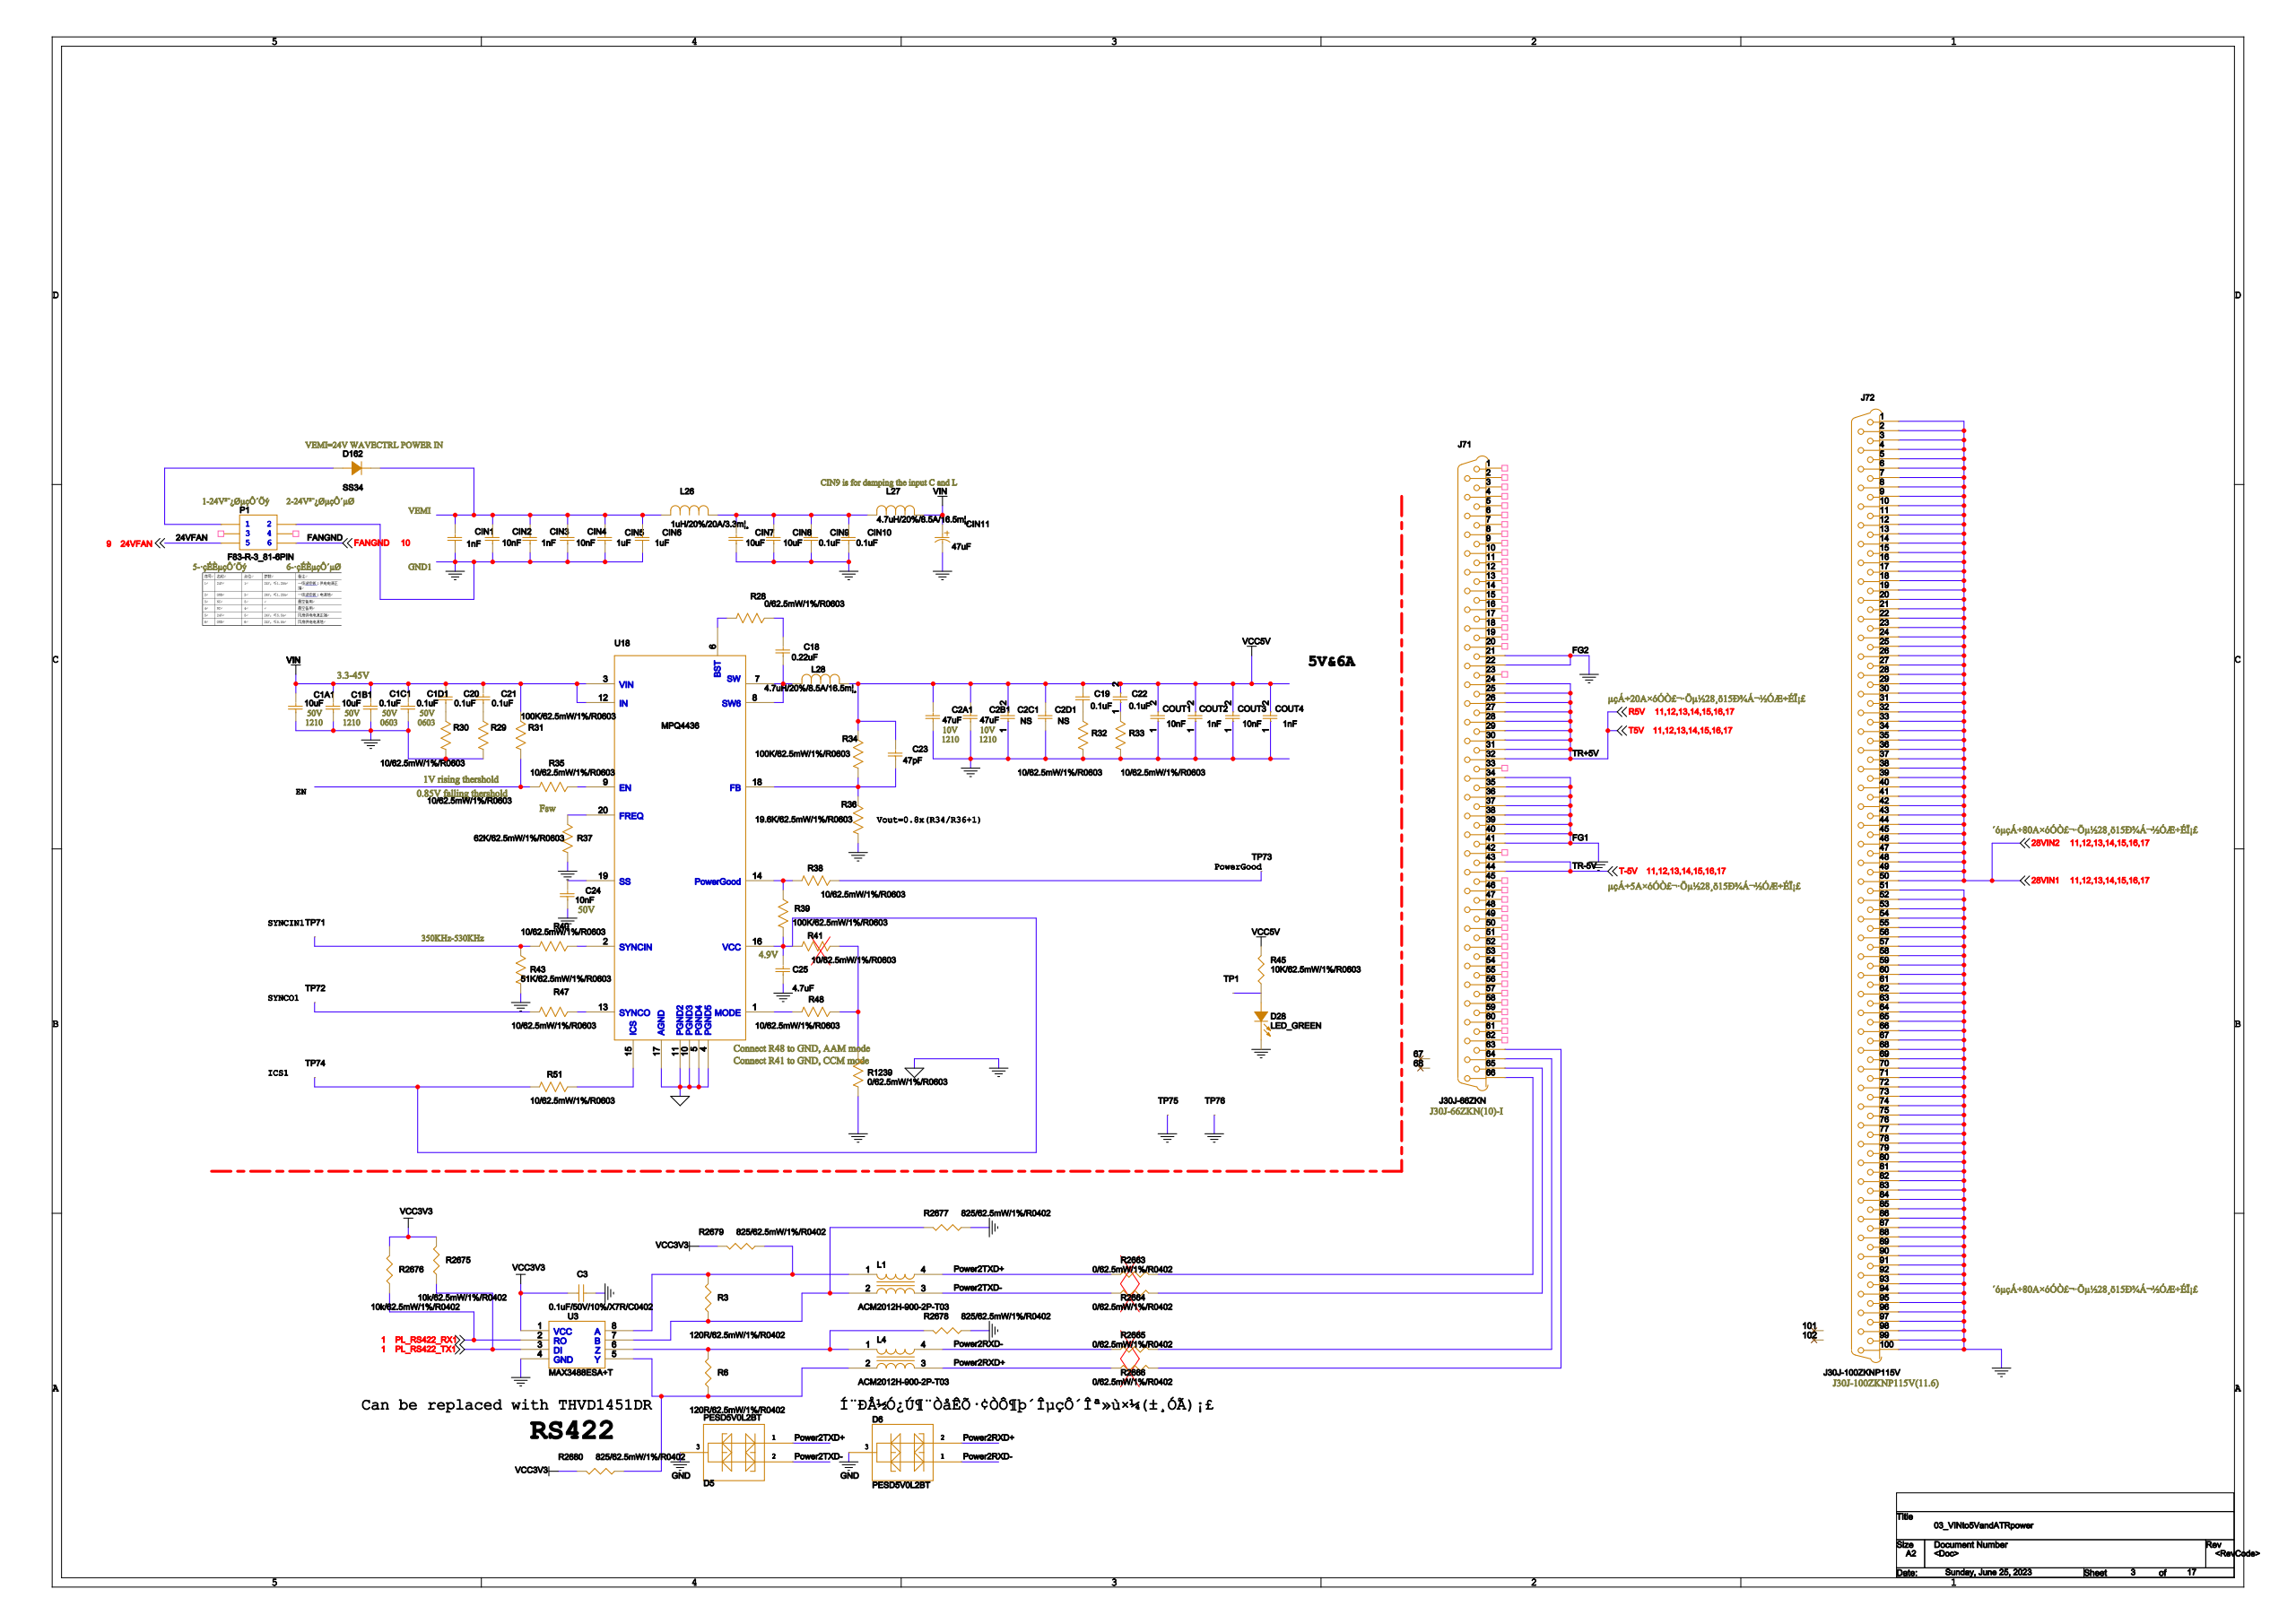Circuit board | Cadence Allegro | 2002 parts | 1538 nets | one sheet of the schematic
Parts on this sheet (reference | value | footprint):
C1A1 | CAP/1210 | 1210
C1B1 | CAP/1210 | 1210
C1C1 | CAP/0603 | 0603C
C1D1 | CAP/0603 | 0603C
C2A1 | CAP/1210 | 1210
C2B1 | CAP/1210 | 1210
C2C1 | CAP/0603 | 0603C
C2D1 | CAP/0603 | 0603C
C3 | 0.1uF/50V/10%/X7R/C0402 | 0402
C18 | CAP/0603 | 0603C
C19 | CAP/0603 | 0603C
C20 | CAP/0603 | 0603C
C21 | CAP/0603 | 0603C
C22 | CAP/0603 | 0603C
C23 | CAP/0603 | 0603C
C24 | CAP/0603 | 0603C
C25 | CAP/0603 | 0603C
CIN1 | CAP/0603 | 0603C
CIN2 | CAP/0603 | 0603C
CIN3 | CAP/0603 | 0603C
CIN4 | CAP/0603 | 0603C
CIN5 | CAP/0603 | 0805C
CIN6 | CAP/0603 | 0805C
CIN7 | CAP/0603 | 1206
CIN8 | CAP/0603 | 1206
CIN9 | CAP/0603 | 0603C
CIN10 | CAP/0603 | 0603C
CIN11 | CAP/ELECT/DIP/OD5.3P2.0 | AP-SMD_BD6_3-L6_6-W6_6-LS7_21
COUT1 | CAP/0603 | 0603C
COUT2 | CAP/0603 | 0603C
COUT3 | CAP/0603 | 0603C
COUT4 | CAP/0603 | 0603C
D5 | PESD5V0L2BT | SOT23
D6 | PESD5V0L2BT | SOT23
D28 | LED_GREEN | LED0805
D162 | SS34 | DO-214AC
J71 | J30J-66ZKN | J30J-66ZKN-I
J72 | J30J-100ZKNP115V | J30J-100ZKNP115V
L1 | ACM2012H-900-2P-T03 | ACM2012
L4 | ACM2012H-900-2P-T03 | ACM2012
L26 | CKST1004-1uH/M-B | SMD_10X11
L27 | CKST1004-4.7uH/M | SMD_10X11
L28 | CKST1004-4.7uH/M | SMD_10X11
P1 | F83-R-3_81-6PIN | F83-R-3_81-6PIN
R3 | 120R/62.5mW/1%/R0402 | 0402
R6 | 120R/62.5mW/1%/R0402 | 0402
R28 | 0/62.5mW/1%/R0603 | 0603R
R29 | 10/62.5mW/1%/R0603 | 0603R
R30 | 10/62.5mW/1%/R0603 | 0603R
R31 | 100K/62.5mW/1%/R0603 | 0603R
R32 | 10/62.5mW/1%/R0603 | 0603R
R33 | 10/62.5mW/1%/R0603 | 0603R
R34 | 100K/62.5mW/1%/R0603 | 0603R
R35 | 10/62.5mW/1%/R0603 | 0603R
R36 | 19.6K/62.5mW/1%/R0603 | 0603R
R37 | 62K/62.5mW/1%/R0603 | 0603R
R38 | 10/62.5mW/1%/R0603 | 0603R
R39 | 100K/62.5mW/1%/R0603 | 0603R
R40 | 10/62.5mW/1%/R0603 | 0603R
R41 | 10/62.5mW/1%/R0603 | 0603R
R43 | 51K/62.5mW/1%/R0603 | 0603R
R45 | 10K/62.5mW/1%/R0603 | 0603R
R47 | 10/62.5mW/1%/R0603 | 0603R
R48 | 10/62.5mW/1%/R0603 | 0603R
R51 | 10/62.5mW/1%/R0603 | 0603R
R1239 | 0/62.5mW/1%/R0603 | 0603R
R2663 | 0/62.5mW/1%/R0402 | 0402
R2664 | 0/62.5mW/1%/R0402 | 0402
R2665 | 0/62.5mW/1%/R0402 | 0402
R2666 | 0/62.5mW/1%/R0402 | 0402
R2675 | 10K/62.5mW/1%/R0402 | 0402
R2676 | 10K/62.5mW/1%/R0402 | 0402
R2677 | 825/62.5mW/1%/R0402 | 0402
R2678 | 825/62.5mW/1%/R0402 | 0402
R2679 | 825/62.5mW/1%/R0402 | 0402
R2680 | 825/62.5mW/1%/R0402 | 0402
TP1 | TEST POINT A | TEST_12MM
TP71 | TEST POINT A | TEST_12MM
TP72 | TEST POINT A | TEST_12MM
TP73 | TEST POINT A | TEST_12MM
TP74 | TEST POINT A | TEST_12MM
TP75 | TEST POINT A | TEST_1MM
TP76 | TEST POINT A | TEST_1MM
U3 | MAX3488ESA+T | SO8
U18 | MPQ4436 | QFN-4X4_MPQ4436-AEC1_MNP
Nets of these parts (net: part-pin ...):
3.3V: C3-1 R2675-1 R2676-1 R2679-1 R2680-1 U3-1
AGND: C1A1-2 C1B1-2 C1C1-2 C1D1-2 C2A1-2 C2B1-2 C2C1-1 C2D1-1 C3-2 C24-2 C25-2 CIN1-2 CIN2-2 CIN3-2 CIN4-2 CIN5-2 CIN6-2 CIN7-2 CIN8-2 CIN9-2 CIN10-2 CIN11-2 COUT1-1 COUT2-1 COUT3-1 COUT4-1 D5-3 D6-3 D28-2 P1-2 R29-2 R30-2 R32-2 R33-2 R36-1 R37-2 R43-1 R1239-2 R2677-2 R2678-2 TP75-1 TP76-1 U3-4 U18-4 U18-5 U18-10 U18-11 U18-17 J71-21 J71-22 J71-34 J71-35 J71-36 J71-37 J71-38 J71-39 J71-40 J71-41 J72-51 J72-52 J72-53 J72-54 J72-55 J72-56 J72-57 J72-58 J72-59 J72-60 J72-61 J72-62 J72-63 J72-64 J72-65 J72-66 J72-67 J72-68 J72-69 J72-70 J72-71 J72-72 J72-73 J72-74 J72-75 J72-76 J72-77 J72-78 J72-79 J72-80 J72-81 J72-82 J72-83 J72-84 J72-85 J72-86 J72-87 J72-88 J72-89 J72-90 J72-91 J72-92 J72-93 J72-94 J72-95 J72-96 J72-97 J72-98 J72-99 J72-100
N24466171: L1-2 R3-2 R2677-1 U3-7
N24466175: L4-1 R6-1 R2678-1 U3-6
N24466169: L1-1 R3-1 R2679-2 U3-8
N24466177: L4-2 R6-2 R2680-2 U3-5
PL_RS422_RX1: R2676-2 U3-2
PL_RS422_TX1: R2675-2 U3-3
VCC5V: C2A1-1 C2B1-1 C2C1-2 C2D1-2 C19-2 C22-2 C23-1 COUT1-2 COUT2-2 COUT3-2 COUT4-2 L28-2 R34-2 R45-2
N24466132: D162-1 P1-1
24VFAN: P1-5
FANGND: P1-6
28VIN1: J72-1 J72-2 J72-3 J72-4 J72-5 J72-6 J72-7 J72-8 J72-9 J72-10 J72-11 J72-12 J72-13 J72-14 J72-15 J72-16 J72-17 J72-18 J72-19 J72-20 J72-21 J72-22 J72-23 J72-24 J72-25 J72-26 J72-27 J72-28 J72-29 J72-30 J72-31 J72-32 J72-33 J72-34 J72-35 J72-36 J72-37 J72-38 J72-39 J72-40 J72-41 J72-42 J72-43 J72-44 J72-45 J72-46 J72-47 J72-48 J72-49 J72-50
R5V: J71-24 J71-25 J71-26 J71-27 J71-28 J71-29 J71-30 J71-31 J71-32
T-5V: J71-43 J71-44
N24509889: R2666-2 J71-63
N24509880: R2665-2 J71-64
N24509871: R2664-2 J71-65
N24509862: R2663-2 J71-66
N24466032: CIN1-1 CIN2-1 CIN3-1 CIN4-1 CIN5-1 CIN6-1 D162-2 L26-1
N24466071: R28-1 U18-6
N24466067: R35-2 U18-9
N24466078: C23-2 R34-1 R36-2 U18-18
N24466030: R37-1 U18-20
N24466058: R51-1 U18-15
VIN: C1A1-1 C1B1-1 C1C1-1 C1D1-1 C20-1 C21-1 CIN11-1 L27-2 R31-2 U18-3 U18-12
N24466061: R48-2 U18-1
N24466062: R38-2 R39-2 U18-14
N24466029: C24-1 U18-19
N24466075: C18-2 L28-1 U18-7 U18-8
N24466031: R40-2 U18-2
N24466056: R47-2 U18-13
N24466060: C25-1 R39-1 R41-2 R51-2 TP74-1 U18-16
N24466073: C18-1 R28-2
N245324920: C19-1 R32-1
N245319080: C20-2 R30-1
N245317461: C21-2 R29-1
N24466125: C22-1 R33-1
N24466045: CIN7-1 CIN8-1 CIN9-1 CIN10-1 L26-2 L27-1
N24466065: R41-1 R48-1 R1239-1
N24466068: R31-1 R35-1
N24466106: R38-1 TP73-1
N24466054: R40-1 R43-2 TP71-1
N24466131: D28-1 R45-1 TP1-1
N24466057: R47-1 TP72-1
POWER2TXD+: D5-1 L1-4 R2663-1
POWER2TXD-: D5-2 L1-3 R2664-1
POWER2RXD-: D6-1 L4-4 R2665-1
POWER2RXD+: D6-2 L4-3 R2666-1